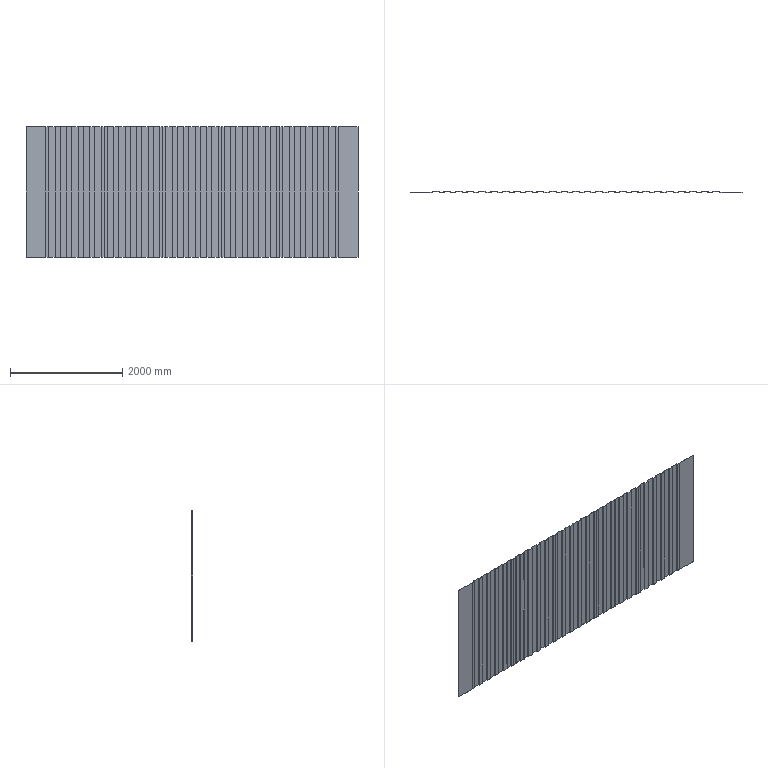Part | SolidWorks | features ICE 2, Extrusion 1, LPattern 1 | 7 solids | 342 faces | box 5925 x 22 x 2324 mm | volume 31788412 mm3 | plane 242 | cylinder 100 | commonest cylinder face diameters 6 x50 10 x50